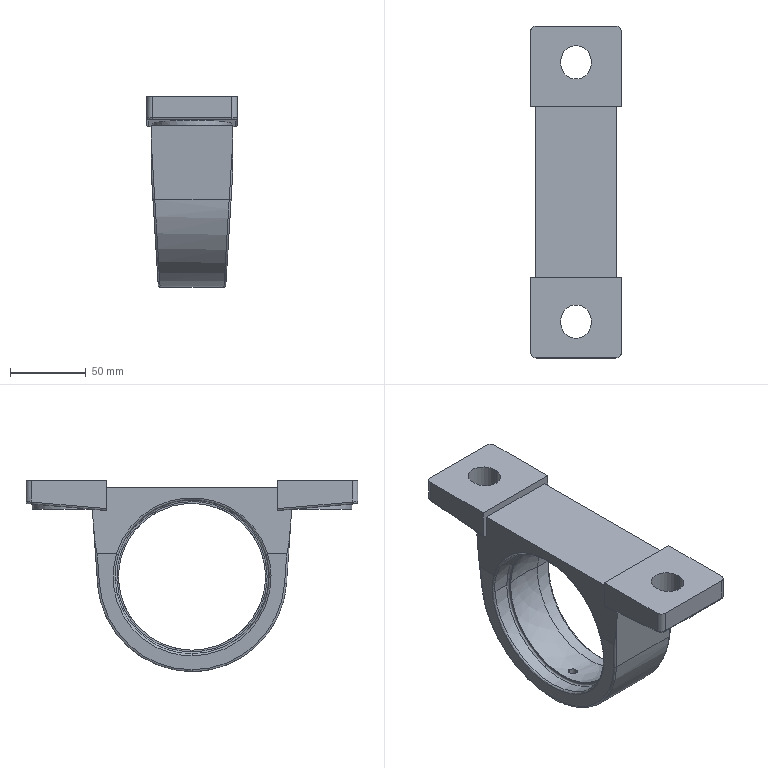Part | STEP file | HOUSE-UCP-211-KONTIMA_UCP_211-K | 1 solid | 76 faces | box 60 x 219 x 126 mm | volume 386400 mm3 | plane 31 | cylinder 27 | spline 10 | torus 6 | sphere 2 | commonest cylinder face diameters 2.533 x10 7.6 x4 20 x4 101.7 x4 6 x2 52.138 x2